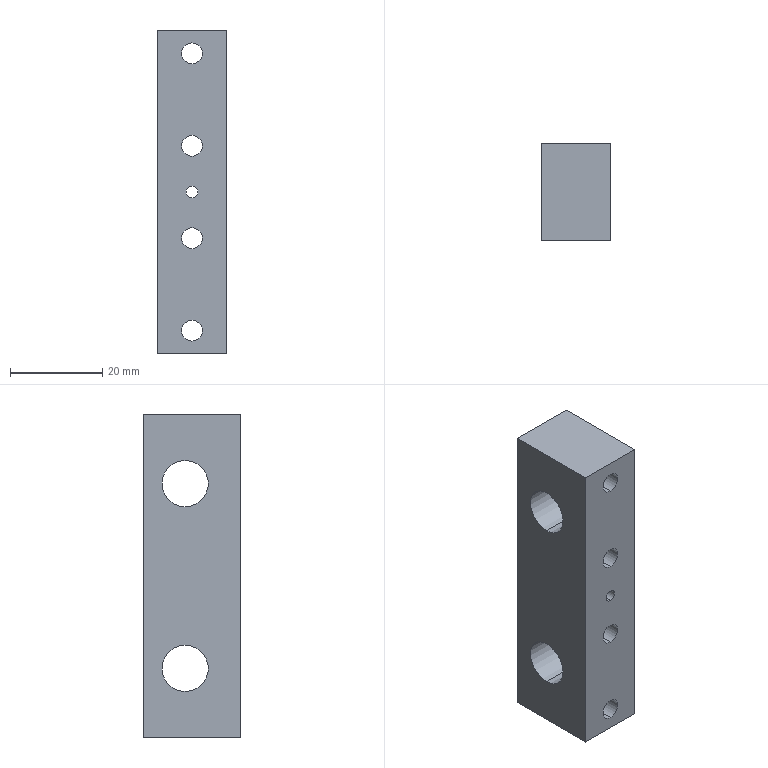Part | STEP file | 0246_204_Block | 1 solid | 32 faces | box 15 x 21 x 70 mm | volume 17430 mm3 | cylinder 22 | plane 10 | commonest cylinder face diameters 4.5 x8 8 x8 10 x4 2.5 x2